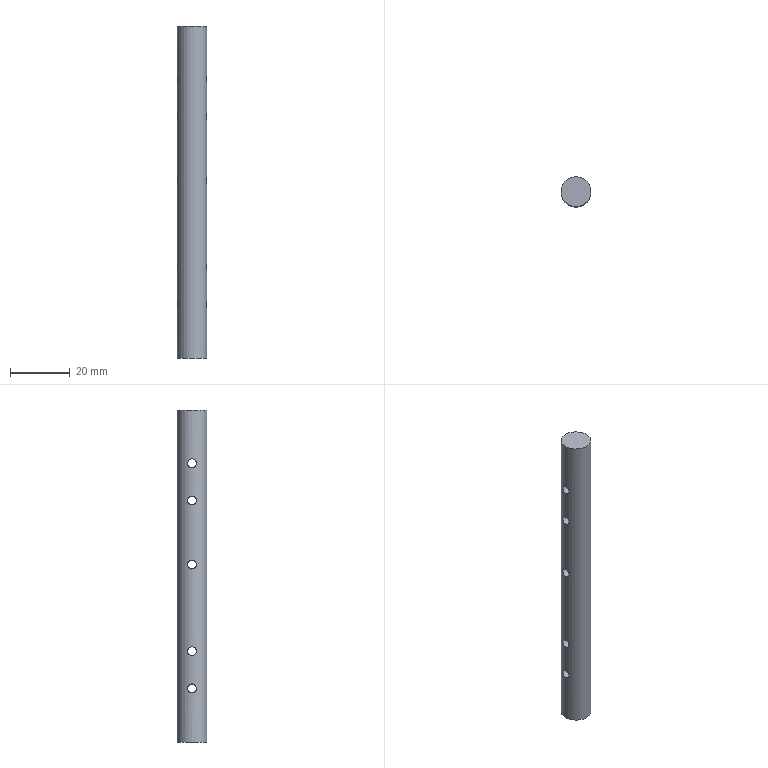Part | NX | features DATUM_CSYS 3, EXTRUDE 2, SKETCH 2, SUBTRACT 1 | 1 solid | 8 faces | box 10 x 10 x 111.5 mm | volume 8408 mm3 | cylinder 6 | plane 2 | commonest cylinder face diameters 3 x5 10 x1
STEP:
#1=CARTESIAN_POINT('',(25.,-0.00001672,57.1));
#2=VERTEX_POINT('',#1);
#3=CARTESIAN_POINT('',(25.113,1.176,56.775));
#4=CARTESIAN_POINT('',(24.944,-0.0001255,57.263));
#5=CARTESIAN_POINT('',(25.113,-1.176,56.774));
#6=CARTESIAN_POINT('',(25.289,-1.662,55.602));
#7=CARTESIAN_POINT('',(25.112,-1.175,54.424));
#8=CARTESIAN_POINT('',(24.944,-0.0008803,53.938));
#9=CARTESIAN_POINT('',(25.112,1.175,54.424));
#10=CARTESIAN_POINT('',(25.289,1.662,55.6));
#11=CARTESIAN_POINT('',(25.113,1.176,56.775));
#12=CARTESIAN_POINT('',(24.944,-0.0001255,57.263));
#13=CARTESIAN_POINT('',(25.113,-1.176,56.774));
#14=B_SPLINE_CURVE_WITH_KNOTS('',3,(#3,#4,#5,#6,#7,#8,#9,#10,#11,#12,#13),.UNSPECIFIED.,.T.,.F.,(1,1,1,1,1,1,1,1,1,1,1,1,1,1,1),(-0.003537,-0.002358,-0.001179,0.,0.001179,0.002358,0.003537,0.004716,0.005895,0.007075,0.008254,0.009433,0.01061,0.01179,0.01297),.UNSPECIFIED.);
#15=EDGE_CURVE('',#2,#2,#14,.T.);
#16=ORIENTED_EDGE('',*,*,#15,.T.);
#17=EDGE_LOOP('',(#16));
#18=FACE_BOUND('',#17,.T.);
#19=CARTESIAN_POINT('',(35.,0.000000625,54.1));
#20=VERTEX_POINT('',#19);
#21=CARTESIAN_POINT('',(34.887,1.176,54.426));
#22=CARTESIAN_POINT('',(35.056,-0.0001062,53.937));
#23=CARTESIAN_POINT('',(34.887,-1.176,54.426));
#24=CARTESIAN_POINT('',(34.711,-1.662,55.598));
#25=CARTESIAN_POINT('',(34.888,-1.175,56.776));
#26=CARTESIAN_POINT('',(35.056,-0.0008996,57.262));
#27=CARTESIAN_POINT('',(34.888,1.175,56.776));
#28=CARTESIAN_POINT('',(34.711,1.662,55.6));
#29=CARTESIAN_POINT('',(34.887,1.176,54.426));
#30=CARTESIAN_POINT('',(35.056,-0.0001062,53.937));
#31=CARTESIAN_POINT('',(34.887,-1.176,54.426));
#32=B_SPLINE_CURVE_WITH_KNOTS('',3,(#21,#22,#23,#24,#25,#26,#27,#28,#29,#30,#31),.UNSPECIFIED.,.T.,.F.,(1,1,1,1,1,1,1,1,1,1,1,1,1,1,1),(-0.003537,-0.002358,-0.001179,0.,0.001179,0.002358,0.003537,0.004716,0.005895,0.007075,0.008254,0.009433,0.01061,0.01179,0.01297),.UNSPECIFIED.);
#33=EDGE_CURVE('',#20,#20,#32,.T.);
#34=ORIENTED_EDGE('',*,*,#33,.T.);
#35=EDGE_LOOP('',(#34));
#36=FACE_BOUND('',#35,.T.);
#37=CARTESIAN_POINT('',(25.,-0.00001672,15.5));
#38=VERTEX_POINT('',#37);
#39=CARTESIAN_POINT('',(25.113,1.176,15.175));
#40=CARTESIAN_POINT('',(24.944,-0.0001255,15.663));
#41=CARTESIAN_POINT('',(25.113,-1.176,15.174));
#42=CARTESIAN_POINT('',(25.289,-1.662,14.002));
#43=CARTESIAN_POINT('',(25.112,-1.175,12.824));
#44=CARTESIAN_POINT('',(24.944,-0.0008803,12.338));
#45=CARTESIAN_POINT('',(25.112,1.175,12.824));
#46=CARTESIAN_POINT('',(25.289,1.662,14.));
#47=CARTESIAN_POINT('',(25.113,1.176,15.175));
#48=CARTESIAN_POINT('',(24.944,-0.0001255,15.663));
#49=CARTESIAN_POINT('',(25.113,-1.176,15.174));
#50=B_SPLINE_CURVE_WITH_KNOTS('',3,(#39,#40,#41,#42,#43,#44,#45,#46,#47,#48,#49),.UNSPECIFIED.,.T.,.F.,(1,1,1,1,1,1,1,1,1,1,1,1,1,1,1),(-0.003537,-0.002358,-0.001179,0.,0.001179,0.002358,0.003537,0.004716,0.005895,0.007075,0.008254,0.009433,0.01061,0.01179,0.01297),.UNSPECIFIED.);
#51=EDGE_CURVE('',#38,#38,#50,.T.);
#52=ORIENTED_EDGE('',*,*,#51,.T.);
#53=EDGE_LOOP('',(#52));
#54=FACE_BOUND('',#53,.T.);
#55=CARTESIAN_POINT('',(35.,0.000000625,12.5));
#56=VERTEX_POINT('',#55);
#57=CARTESIAN_POINT('',(34.887,1.176,12.826));
#58=CARTESIAN_POINT('',(35.056,-0.0001062,12.337));
#59=CARTESIAN_POINT('',(34.887,-1.176,12.826));
#60=CARTESIAN_POINT('',(34.711,-1.662,13.998));
#61=CARTESIAN_POINT('',(34.888,-1.175,15.176));
#62=CARTESIAN_POINT('',(35.056,-0.0008996,15.662));
#63=CARTESIAN_POINT('',(34.888,1.175,15.176));
#64=CARTESIAN_POINT('',(34.711,1.662,14.));
#65=CARTESIAN_POINT('',(34.887,1.176,12.826));
#66=CARTESIAN_POINT('',(35.056,-0.0001062,12.337));
#67=CARTESIAN_POINT('',(34.887,-1.176,12.826));
#68=B_SPLINE_CURVE_WITH_KNOTS('',3,(#57,#58,#59,#60,#61,#62,#63,#64,#65,#66,#67),.UNSPECIFIED.,.T.,.F.,(1,1,1,1,1,1,1,1,1,1,1,1,1,1,1),(-0.003537,-0.002358,-0.001179,0.,0.001179,0.002358,0.003537,0.004716,0.005895,0.007075,0.008254,0.009433,0.01061,0.01179,0.01297),.UNSPECIFIED.);
#69=EDGE_CURVE('',#56,#56,#68,.T.);
#70=ORIENTED_EDGE('',*,*,#69,.T.);
#71=EDGE_LOOP('',(#70));
#72=FACE_BOUND('',#71,.T.);
#73=CARTESIAN_POINT('',(35.,-0.00001672,107.5));
#74=VERTEX_POINT('',#73);
#75=CARTESIAN_POINT('',(30.,-0.00001672,107.5));
#76=DIRECTION('',(0.,0.,1.));
#77=DIRECTION('',(1.,0.,0.));
#78=AXIS2_PLACEMENT_3D('',#75,#76,#77);
#79=CIRCLE('',#78,5.);
#80=EDGE_CURVE('',#74,#74,#79,.T.);
#81=ORIENTED_EDGE('',*,*,#80,.F.);
#82=EDGE_LOOP('',(#81));
#83=FACE_BOUND('',#82,.T.);
#84=CARTESIAN_POINT('',(35.,-0.00001672,-4.));
#85=VERTEX_POINT('',#84);
#86=CARTESIAN_POINT('',(30.,-0.00001672,-4.));
#87=DIRECTION('',(0.,0.,1.));
#88=DIRECTION('',(1.,0.,0.));
#89=AXIS2_PLACEMENT_3D('',#86,#87,#88);
#90=CIRCLE('',#89,5.);
#91=EDGE_CURVE('',#85,#85,#90,.T.);
#92=ORIENTED_EDGE('',*,*,#91,.T.);
#93=EDGE_LOOP('',(#92));
#94=FACE_BOUND('',#93,.T.);
#95=CARTESIAN_POINT('',(35.,0.000000625,25.));
#96=VERTEX_POINT('',#95);
#97=CARTESIAN_POINT('',(34.887,-1.176,25.326));
#98=CARTESIAN_POINT('',(35.056,0.0001078,24.837));
#99=CARTESIAN_POINT('',(34.887,1.176,25.326));
#100=CARTESIAN_POINT('',(34.711,1.662,26.498));
#101=CARTESIAN_POINT('',(34.888,1.175,27.676));
#102=CARTESIAN_POINT('',(35.056,0.0009038,28.162));
#103=CARTESIAN_POINT('',(34.888,-1.175,27.676));
#104=CARTESIAN_POINT('',(34.711,-1.662,26.5));
#105=CARTESIAN_POINT('',(34.887,-1.176,25.326));
#106=CARTESIAN_POINT('',(35.056,0.0001078,24.837));
#107=CARTESIAN_POINT('',(34.887,1.176,25.326));
#108=B_SPLINE_CURVE_WITH_KNOTS('',3,(#97,#98,#99,#100,#101,#102,#103,#104,#105,#106,#107),.UNSPECIFIED.,.T.,.F.,(1,1,1,1,1,1,1,1,1,1,1,1,1,1,1),(-0.003537,-0.002358,-0.001179,0.,0.001179,0.002358,0.003537,0.004716,0.005895,0.007075,0.008254,0.009433,0.01061,0.01179,0.01297),.UNSPECIFIED.);
#109=EDGE_CURVE('',#96,#96,#108,.T.);
#110=ORIENTED_EDGE('',*,*,#109,.F.);
#111=EDGE_LOOP('',(#110));
#112=FACE_BOUND('',#111,.T.);
#113=CARTESIAN_POINT('',(25.,-0.00001672,28.));
#114=VERTEX_POINT('',#113);
#115=CARTESIAN_POINT('',(25.113,-1.176,27.675));
#116=CARTESIAN_POINT('',(24.944,0.00008848,28.163));
#117=CARTESIAN_POINT('',(25.113,1.176,27.674));
#118=CARTESIAN_POINT('',(25.289,1.662,26.502));
#119=CARTESIAN_POINT('',(25.112,1.175,25.324));
#120=CARTESIAN_POINT('',(24.944,0.0009231,24.838));
#121=CARTESIAN_POINT('',(25.112,-1.175,25.324));
#122=CARTESIAN_POINT('',(25.289,-1.662,26.5));
#123=CARTESIAN_POINT('',(25.113,-1.176,27.675));
#124=CARTESIAN_POINT('',(24.944,0.00008848,28.163));
#125=CARTESIAN_POINT('',(25.113,1.176,27.674));
#126=B_SPLINE_CURVE_WITH_KNOTS('',3,(#115,#116,#117,#118,#119,#120,#121,#122,#123,#124,#125),.UNSPECIFIED.,.T.,.F.,(1,1,1,1,1,1,1,1,1,1,1,1,1,1,1),(-0.003537,-0.002358,-0.001179,0.,0.001179,0.002358,0.003537,0.004716,0.005895,0.007075,0.008254,0.009433,0.01061,0.01179,0.01297),.UNSPECIFIED.);
#127=EDGE_CURVE('',#114,#114,#126,.T.);
#128=ORIENTED_EDGE('',*,*,#127,.F.);
#129=EDGE_LOOP('',(#128));
#130=FACE_BOUND('',#129,.T.);
#131=CARTESIAN_POINT('',(35.,0.000000625,75.6));
#132=VERTEX_POINT('',#131);
#133=CARTESIAN_POINT('',(34.887,-1.176,75.926));
#134=CARTESIAN_POINT('',(35.056,0.0001078,75.437));
#135=CARTESIAN_POINT('',(34.887,1.176,75.926));
#136=CARTESIAN_POINT('',(34.711,1.662,77.098));
#137=CARTESIAN_POINT('',(34.888,1.175,78.276));
#138=CARTESIAN_POINT('',(35.056,0.0009038,78.762));
#139=CARTESIAN_POINT('',(34.888,-1.175,78.276));
#140=CARTESIAN_POINT('',(34.711,-1.662,77.1));
#141=CARTESIAN_POINT('',(34.887,-1.176,75.926));
#142=CARTESIAN_POINT('',(35.056,0.0001078,75.437));
#143=CARTESIAN_POINT('',(34.887,1.176,75.926));
#144=B_SPLINE_CURVE_WITH_KNOTS('',3,(#133,#134,#135,#136,#137,#138,#139,#140,#141,#142,#143),.UNSPECIFIED.,.T.,.F.,(1,1,1,1,1,1,1,1,1,1,1,1,1,1,1),(-0.003537,-0.002358,-0.001179,0.,0.001179,0.002358,0.003537,0.004716,0.005895,0.007075,0.008254,0.009433,0.01061,0.01179,0.01297),.UNSPECIFIED.);
#145=EDGE_CURVE('',#132,#132,#144,.T.);
#146=ORIENTED_EDGE('',*,*,#145,.F.);
#147=EDGE_LOOP('',(#146));
#148=FACE_BOUND('',#147,.T.);
#149=CARTESIAN_POINT('',(25.,-0.00001672,78.6));
#150=VERTEX_POINT('',#149);
#151=CARTESIAN_POINT('',(25.113,-1.176,78.275));
#152=CARTESIAN_POINT('',(24.944,0.00008848,78.763));
#153=CARTESIAN_POINT('',(25.113,1.176,78.274));
#154=CARTESIAN_POINT('',(25.289,1.662,77.102));
#155=CARTESIAN_POINT('',(25.112,1.175,75.924));
#156=CARTESIAN_POINT('',(24.944,0.0009231,75.438));
#157=CARTESIAN_POINT('',(25.112,-1.175,75.924));
#158=CARTESIAN_POINT('',(25.289,-1.662,77.1));
#159=CARTESIAN_POINT('',(25.113,-1.176,78.275));
#160=CARTESIAN_POINT('',(24.944,0.00008848,78.763));
#161=CARTESIAN_POINT('',(25.113,1.176,78.274));
#162=B_SPLINE_CURVE_WITH_KNOTS('',3,(#151,#152,#153,#154,#155,#156,#157,#158,#159,#160,#161),.UNSPECIFIED.,.T.,.F.,(1,1,1,1,1,1,1,1,1,1,1,1,1,1,1),(-0.003537,-0.002358,-0.001179,0.,0.001179,0.002358,0.003537,0.004716,0.005895,0.007075,0.008254,0.009433,0.01061,0.01179,0.01297),.UNSPECIFIED.);
#163=EDGE_CURVE('',#150,#150,#162,.T.);
#164=ORIENTED_EDGE('',*,*,#163,.F.);
#165=EDGE_LOOP('',(#164));
#166=FACE_BOUND('',#165,.T.);
#167=CARTESIAN_POINT('',(35.,0.000000625,88.1));
#168=VERTEX_POINT('',#167);
#169=CARTESIAN_POINT('',(34.887,-1.176,88.426));
#170=CARTESIAN_POINT('',(35.056,0.0001078,87.937));
#171=CARTESIAN_POINT('',(34.887,1.176,88.426));
#172=CARTESIAN_POINT('',(34.711,1.662,89.598));
#173=CARTESIAN_POINT('',(34.888,1.175,90.776));
#174=CARTESIAN_POINT('',(35.056,0.0009038,91.262));
#175=CARTESIAN_POINT('',(34.888,-1.175,90.776));
#176=CARTESIAN_POINT('',(34.711,-1.662,89.6));
#177=CARTESIAN_POINT('',(34.887,-1.176,88.426));
#178=CARTESIAN_POINT('',(35.056,0.0001078,87.937));
#179=CARTESIAN_POINT('',(34.887,1.176,88.426));
#180=B_SPLINE_CURVE_WITH_KNOTS('',3,(#169,#170,#171,#172,#173,#174,#175,#176,#177,#178,#179),.UNSPECIFIED.,.T.,.F.,(1,1,1,1,1,1,1,1,1,1,1,1,1,1,1),(-0.003537,-0.002358,-0.001179,0.,0.001179,0.002358,0.003537,0.004716,0.005895,0.007075,0.008254,0.009433,0.01061,0.01179,0.01297),.UNSPECIFIED.);
#181=EDGE_CURVE('',#168,#168,#180,.T.);
#182=ORIENTED_EDGE('',*,*,#181,.F.);
#183=EDGE_LOOP('',(#182));
#184=FACE_BOUND('',#183,.T.);
#185=CARTESIAN_POINT('',(25.,-0.00001672,91.1));
#186=VERTEX_POINT('',#185);
#187=CARTESIAN_POINT('',(25.113,-1.176,90.775));
#188=CARTESIAN_POINT('',(24.944,0.00008848,91.263));
#189=CARTESIAN_POINT('',(25.113,1.176,90.774));
#190=CARTESIAN_POINT('',(25.289,1.662,89.602));
#191=CARTESIAN_POINT('',(25.112,1.175,88.424));
#192=CARTESIAN_POINT('',(24.944,0.0009231,87.938));
#193=CARTESIAN_POINT('',(25.112,-1.175,88.424));
#194=CARTESIAN_POINT('',(25.289,-1.662,89.6));
#195=CARTESIAN_POINT('',(25.113,-1.176,90.775));
#196=CARTESIAN_POINT('',(24.944,0.00008848,91.263));
#197=CARTESIAN_POINT('',(25.113,1.176,90.774));
#198=B_SPLINE_CURVE_WITH_KNOTS('',3,(#187,#188,#189,#190,#191,#192,#193,#194,#195,#196,#197),.UNSPECIFIED.,.T.,.F.,(1,1,1,1,1,1,1,1,1,1,1,1,1,1,1),(-0.003537,-0.002358,-0.001179,0.,0.001179,0.002358,0.003537,0.004716,0.005895,0.007075,0.008254,0.009433,0.01061,0.01179,0.01297),.UNSPECIFIED.);
#199=EDGE_CURVE('',#186,#186,#198,.T.);
#200=ORIENTED_EDGE('',*,*,#199,.F.);
#201=EDGE_LOOP('',(#200));
#202=FACE_BOUND('',#201,.T.);
#203=CARTESIAN_POINT('',(30.,-0.00001672,107.5));
#204=DIRECTION('',(0.,0.,-1.));
#205=DIRECTION('',(-1.,0.,0.));
#206=AXIS2_PLACEMENT_3D('',#203,#204,#205);
#207=CYLINDRICAL_SURFACE('',#206,5.);
#208=ADVANCED_FACE('',(#18,#36,#54,#72,#83,#94,#112,#130,#148,#166,#184,#202),#207,.T.);
#209=ORIENTED_EDGE('',*,*,#80,.T.);
#210=EDGE_LOOP('',(#209));
#211=FACE_BOUND('',#210,.T.);
#212=CARTESIAN_POINT('',(30.,-0.00001672,107.5));
#213=DIRECTION('',(0.,0.,1.));
#214=DIRECTION('',(1.,0.,0.));
#215=AXIS2_PLACEMENT_3D('',#212,#213,#214);
#216=PLANE('',#215);
#217=ADVANCED_FACE('',(#211),#216,.T.);
#218=ORIENTED_EDGE('',*,*,#91,.F.);
#219=EDGE_LOOP('',(#218));
#220=FACE_BOUND('',#219,.T.);
#221=CARTESIAN_POINT('',(30.,-0.00001672,-4.));
#222=DIRECTION('',(0.,0.,1.));
#223=DIRECTION('',(1.,0.,0.));
#224=AXIS2_PLACEMENT_3D('',#221,#222,#223);
#225=PLANE('',#224);
#226=ADVANCED_FACE('',(#220),#225,.F.);
#227=ORIENTED_EDGE('',*,*,#69,.F.);
#228=EDGE_LOOP('',(#227));
#229=FACE_BOUND('',#228,.T.);
#230=ORIENTED_EDGE('',*,*,#51,.F.);
#231=EDGE_LOOP('',(#230));
#232=FACE_BOUND('',#231,.T.);
#233=CARTESIAN_POINT('',(-32.,0.000000625,14.));
#234=DIRECTION('',(1.,0.,0.));
#235=DIRECTION('',(0.,0.,-1.));
#236=AXIS2_PLACEMENT_3D('',#233,#234,#235);
#237=CYLINDRICAL_SURFACE('',#236,1.5);
#238=ADVANCED_FACE('',(#229,#232),#237,.F.);
#239=ORIENTED_EDGE('',*,*,#109,.T.);
#240=EDGE_LOOP('',(#239));
#241=FACE_BOUND('',#240,.T.);
#242=ORIENTED_EDGE('',*,*,#127,.T.);
#243=EDGE_LOOP('',(#242));
#244=FACE_BOUND('',#243,.T.);
#245=CARTESIAN_POINT('',(-32.,0.000000625,26.5));
#246=DIRECTION('',(1.,0.,0.));
#247=DIRECTION('',(0.,0.,-1.));
#248=AXIS2_PLACEMENT_3D('',#245,#246,#247);
#249=CYLINDRICAL_SURFACE('',#248,1.5);
#250=ADVANCED_FACE('',(#241,#244),#249,.F.);
#251=ORIENTED_EDGE('',*,*,#33,.F.);
#252=EDGE_LOOP('',(#251));
#253=FACE_BOUND('',#252,.T.);
#254=ORIENTED_EDGE('',*,*,#15,.F.);
#255=EDGE_LOOP('',(#254));
#256=FACE_BOUND('',#255,.T.);
#257=CARTESIAN_POINT('',(-32.,0.000000625,55.6));
#258=DIRECTION('',(1.,0.,0.));
#259=DIRECTION('',(0.,0.,-1.));
#260=AXIS2_PLACEMENT_3D('',#257,#258,#259);
#261=CYLINDRICAL_SURFACE('',#260,1.5);
#262=ADVANCED_FACE('',(#253,#256),#261,.F.);
#263=ORIENTED_EDGE('',*,*,#145,.T.);
#264=EDGE_LOOP('',(#263));
#265=FACE_BOUND('',#264,.T.);
#266=ORIENTED_EDGE('',*,*,#163,.T.);
#267=EDGE_LOOP('',(#266));
#268=FACE_BOUND('',#267,.T.);
#269=CARTESIAN_POINT('',(-32.,0.000000625,77.1));
#270=DIRECTION('',(1.,0.,0.));
#271=DIRECTION('',(0.,0.,-1.));
#272=AXIS2_PLACEMENT_3D('',#269,#270,#271);
#273=CYLINDRICAL_SURFACE('',#272,1.5);
#274=ADVANCED_FACE('',(#265,#268),#273,.F.);
#275=ORIENTED_EDGE('',*,*,#181,.T.);
#276=EDGE_LOOP('',(#275));
#277=FACE_BOUND('',#276,.T.);
#278=ORIENTED_EDGE('',*,*,#199,.T.);
#279=EDGE_LOOP('',(#278));
#280=FACE_BOUND('',#279,.T.);
#281=CARTESIAN_POINT('',(-32.,0.000000625,89.6));
#282=DIRECTION('',(1.,0.,0.));
#283=DIRECTION('',(0.,0.,-1.));
#284=AXIS2_PLACEMENT_3D('',#281,#282,#283);
#285=CYLINDRICAL_SURFACE('',#284,1.5);
#286=ADVANCED_FACE('',(#277,#280),#285,.F.);
#287=CLOSED_SHELL('',(#208,#217,#226,#238,#250,#262,#274,#286));
#288=MANIFOLD_SOLID_BREP('',#287);
#289=(LENGTH_UNIT()NAMED_UNIT(*)SI_UNIT(.MILLI.,.METRE.));
#290=UNCERTAINTY_MEASURE_WITH_UNIT(LENGTH_MEASURE(0.0508),#289,'','');
#291=(NAMED_UNIT(*)PLANE_ANGLE_UNIT()SI_UNIT($,.RADIAN.));
#292=(NAMED_UNIT(*)SI_UNIT($,.STERADIAN.)SOLID_ANGLE_UNIT());
#293=(GEOMETRIC_REPRESENTATION_CONTEXT(3)GLOBAL_UNCERTAINTY_ASSIGNED_CONTEXT((#290))GLOBAL_UNIT_ASSIGNED_CONTEXT((#289,#291,#292))REPRESENTATION_CONTEXT('',''));
#294=ADVANCED_BREP_SHAPE_REPRESENTATION('',(#288),#293);